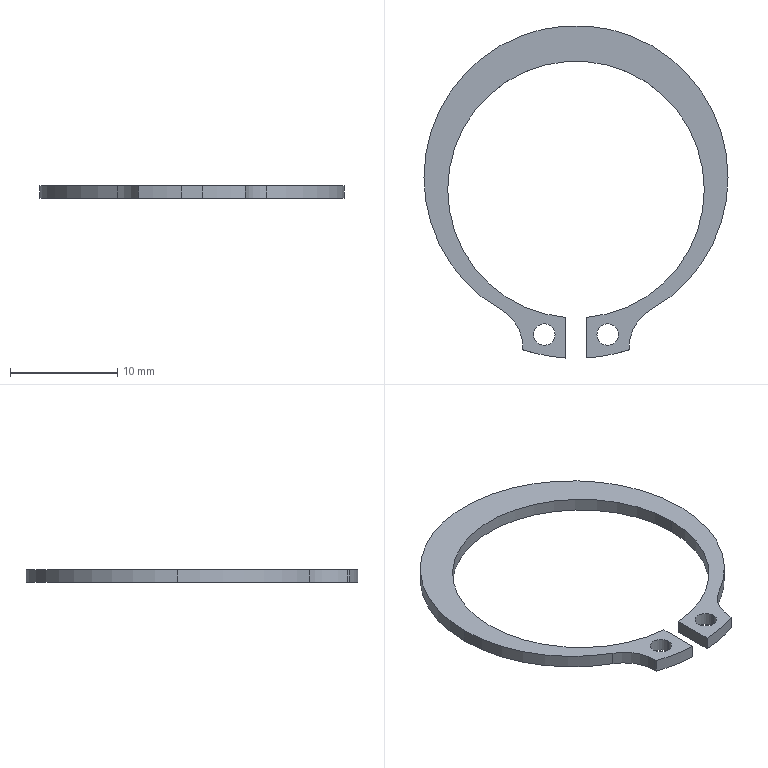Part | SolidWorks | features BaseBody 1 | 1 solid | 20 faces | box 28.327 x 30.963 x 1.2 mm | volume 236.217 mm3 | cylinder 14 | plane 6 | commonest cylinder face diameters 2 x4 23.9 x3 28.327 x3 8 x2 31.443 x2
STEP:
#1=CARTESIAN_POINT('',(4.9,-1.605,1.2));
#2=VERTEX_POINT('',#1);
#3=CARTESIAN_POINT('',(2.9,-1.605,1.2));
#4=VERTEX_POINT('',#3);
#5=CARTESIAN_POINT('',(3.9,-1.605,1.2));
#6=DIRECTION('',(0.,0.,-1.));
#7=DIRECTION('',(-1.,0.,0.));
#8=AXIS2_PLACEMENT_3D('',#5,#6,#7);
#9=CIRCLE('',#8,1.);
#10=EDGE_CURVE('',#2,#4,#9,.T.);
#11=ORIENTED_EDGE('',*,*,#10,.F.);
#12=CARTESIAN_POINT('',(4.9,-1.605,0.));
#13=VERTEX_POINT('',#12);
#14=CARTESIAN_POINT('',(4.9,-1.605,1.2));
#15=DIRECTION('',(0.,0.,-1.));
#16=VECTOR('',#15,1000.);
#17=LINE('',#14,#16);
#18=EDGE_CURVE('',#2,#13,#17,.T.);
#19=ORIENTED_EDGE('',*,*,#18,.T.);
#20=CARTESIAN_POINT('',(2.9,-1.605,0.));
#21=VERTEX_POINT('',#20);
#22=CARTESIAN_POINT('',(3.9,-1.605,0.));
#23=DIRECTION('',(0.,0.,-1.));
#24=DIRECTION('',(-1.,0.,0.));
#25=AXIS2_PLACEMENT_3D('',#22,#23,#24);
#26=CIRCLE('',#25,1.);
#27=EDGE_CURVE('',#13,#21,#26,.T.);
#28=ORIENTED_EDGE('',*,*,#27,.T.);
#29=CARTESIAN_POINT('',(2.9,-1.605,1.2));
#30=DIRECTION('',(0.,0.,-1.));
#31=VECTOR('',#30,1000.);
#32=LINE('',#29,#31);
#33=EDGE_CURVE('',#4,#21,#32,.T.);
#34=ORIENTED_EDGE('',*,*,#33,.F.);
#35=EDGE_LOOP('',(#11,#19,#28,#34));
#36=FACE_OUTER_BOUND('',#35,.T.);
#37=CARTESIAN_POINT('',(3.9,-1.605,1.2));
#38=DIRECTION('',(0.,0.,-1.));
#39=DIRECTION('',(-1.,0.,0.));
#40=AXIS2_PLACEMENT_3D('',#37,#38,#39);
#41=CYLINDRICAL_SURFACE('',#40,1.);
#42=ADVANCED_FACE('',(#36),#41,.F.);
#43=CARTESIAN_POINT('',(-1.,-1.605,0.));
#44=VERTEX_POINT('',#43);
#45=CARTESIAN_POINT('',(-3.,-1.605,0.));
#46=VERTEX_POINT('',#45);
#47=CARTESIAN_POINT('',(-2.,-1.605,0.));
#48=DIRECTION('',(0.,0.,-1.));
#49=DIRECTION('',(1.,0.,0.));
#50=AXIS2_PLACEMENT_3D('',#47,#48,#49);
#51=CIRCLE('',#50,1.);
#52=EDGE_CURVE('',#44,#46,#51,.T.);
#53=ORIENTED_EDGE('',*,*,#52,.T.);
#54=CARTESIAN_POINT('',(-3.,-1.605,1.2));
#55=VERTEX_POINT('',#54);
#56=CARTESIAN_POINT('',(-3.,-1.605,1.2));
#57=DIRECTION('',(0.,0.,1.));
#58=VECTOR('',#57,1000.);
#59=LINE('',#56,#58);
#60=EDGE_CURVE('',#46,#55,#59,.T.);
#61=ORIENTED_EDGE('',*,*,#60,.T.);
#62=CARTESIAN_POINT('',(-1.,-1.605,1.2));
#63=VERTEX_POINT('',#62);
#64=CARTESIAN_POINT('',(-2.,-1.605,1.2));
#65=DIRECTION('',(0.,0.,-1.));
#66=DIRECTION('',(1.,0.,0.));
#67=AXIS2_PLACEMENT_3D('',#64,#65,#66);
#68=CIRCLE('',#67,1.);
#69=EDGE_CURVE('',#63,#55,#68,.T.);
#70=ORIENTED_EDGE('',*,*,#69,.F.);
#71=CARTESIAN_POINT('',(-1.,-1.605,1.2));
#72=DIRECTION('',(0.,0.,1.));
#73=VECTOR('',#72,1000.);
#74=LINE('',#71,#73);
#75=EDGE_CURVE('',#44,#63,#74,.T.);
#76=ORIENTED_EDGE('',*,*,#75,.F.);
#77=EDGE_LOOP('',(#53,#61,#70,#76));
#78=FACE_OUTER_BOUND('',#77,.T.);
#79=CARTESIAN_POINT('',(-2.,-1.605,1.2));
#80=DIRECTION('',(0.,0.,1.));
#81=DIRECTION('',(1.,0.,0.));
#82=AXIS2_PLACEMENT_3D('',#79,#80,#81);
#83=CYLINDRICAL_SURFACE('',#82,1.);
#84=ADVANCED_FACE('',(#78),#83,.F.);
#85=CARTESIAN_POINT('',(15.113,13.019,0.));
#86=VERTEX_POINT('',#85);
#87=CARTESIAN_POINT('',(-13.213,13.019,0.));
#88=VERTEX_POINT('',#87);
#89=CARTESIAN_POINT('',(0.95,13.019,0.));
#90=DIRECTION('',(0.,0.,1.));
#91=DIRECTION('',(1.,0.,0.));
#92=AXIS2_PLACEMENT_3D('',#89,#90,#91);
#93=CIRCLE('',#92,14.163);
#94=EDGE_CURVE('',#86,#88,#93,.T.);
#95=ORIENTED_EDGE('',*,*,#94,.T.);
#96=CARTESIAN_POINT('',(-13.213,13.019,1.2));
#97=VERTEX_POINT('',#96);
#98=CARTESIAN_POINT('',(-13.213,13.019,0.));
#99=DIRECTION('',(0.,0.,1.));
#100=VECTOR('',#99,1000.);
#101=LINE('',#98,#100);
#102=EDGE_CURVE('',#88,#97,#101,.T.);
#103=ORIENTED_EDGE('',*,*,#102,.T.);
#104=CARTESIAN_POINT('',(15.113,13.019,1.2));
#105=VERTEX_POINT('',#104);
#106=CARTESIAN_POINT('',(0.95,13.019,1.2));
#107=DIRECTION('',(0.,0.,-1.));
#108=DIRECTION('',(1.,0.,0.));
#109=AXIS2_PLACEMENT_3D('',#106,#107,#108);
#110=CIRCLE('',#109,14.163);
#111=EDGE_CURVE('',#97,#105,#110,.T.);
#112=ORIENTED_EDGE('',*,*,#111,.T.);
#113=CARTESIAN_POINT('',(15.113,13.019,0.));
#114=DIRECTION('',(0.,0.,1.));
#115=VECTOR('',#114,1000.);
#116=LINE('',#113,#115);
#117=EDGE_CURVE('',#86,#105,#116,.T.);
#118=ORIENTED_EDGE('',*,*,#117,.F.);
#119=EDGE_LOOP('',(#95,#103,#112,#118));
#120=FACE_OUTER_BOUND('',#119,.T.);
#121=CARTESIAN_POINT('',(0.95,13.019,0.));
#122=DIRECTION('',(0.,0.,1.));
#123=DIRECTION('',(1.,0.,0.));
#124=AXIS2_PLACEMENT_3D('',#121,#122,#123);
#125=CYLINDRICAL_SURFACE('',#124,14.163);
#126=ADVANCED_FACE('',(#120),#125,.T.);
#127=CARTESIAN_POINT('',(7.929,0.6943,0.));
#128=VERTEX_POINT('',#127);
#129=CARTESIAN_POINT('',(0.95,13.019,0.));
#130=DIRECTION('',(0.,0.,1.));
#131=DIRECTION('',(1.,0.,0.));
#132=AXIS2_PLACEMENT_3D('',#129,#130,#131);
#133=CIRCLE('',#132,14.163);
#134=EDGE_CURVE('',#128,#86,#133,.T.);
#135=ORIENTED_EDGE('',*,*,#134,.T.);
#136=ORIENTED_EDGE('',*,*,#117,.T.);
#137=CARTESIAN_POINT('',(7.929,0.6943,1.2));
#138=VERTEX_POINT('',#137);
#139=CARTESIAN_POINT('',(0.95,13.019,1.2));
#140=DIRECTION('',(0.,0.,-1.));
#141=DIRECTION('',(1.,0.,0.));
#142=AXIS2_PLACEMENT_3D('',#139,#140,#141);
#143=CIRCLE('',#142,14.163);
#144=EDGE_CURVE('',#105,#138,#143,.T.);
#145=ORIENTED_EDGE('',*,*,#144,.T.);
#146=CARTESIAN_POINT('',(7.929,0.6943,0.));
#147=DIRECTION('',(0.,0.,-1.));
#148=VECTOR('',#147,1000.);
#149=LINE('',#146,#148);
#150=EDGE_CURVE('',#138,#128,#149,.T.);
#151=ORIENTED_EDGE('',*,*,#150,.T.);
#152=EDGE_LOOP('',(#135,#136,#145,#151));
#153=FACE_OUTER_BOUND('',#152,.T.);
#154=CARTESIAN_POINT('',(0.95,13.019,0.));
#155=DIRECTION('',(0.,0.,1.));
#156=DIRECTION('',(1.,0.,0.));
#157=AXIS2_PLACEMENT_3D('',#154,#155,#156);
#158=CYLINDRICAL_SURFACE('',#157,14.163);
#159=ADVANCED_FACE('',(#153),#158,.T.);
#160=CARTESIAN_POINT('',(0.,0.,0.));
#161=VERTEX_POINT('',#160);
#162=CARTESIAN_POINT('',(-11.,11.912,0.));
#163=VERTEX_POINT('',#162);
#164=CARTESIAN_POINT('',(0.95,11.912,0.));
#165=DIRECTION('',(0.,0.,-1.));
#166=DIRECTION('',(1.,0.,0.));
#167=AXIS2_PLACEMENT_3D('',#164,#165,#166);
#168=CIRCLE('',#167,11.95);
#169=EDGE_CURVE('',#161,#163,#168,.T.);
#170=ORIENTED_EDGE('',*,*,#169,.T.);
#171=CARTESIAN_POINT('',(-11.,11.912,1.2));
#172=VERTEX_POINT('',#171);
#173=CARTESIAN_POINT('',(-11.,11.912,0.));
#174=DIRECTION('',(0.,0.,1.));
#175=VECTOR('',#174,1000.);
#176=LINE('',#173,#175);
#177=EDGE_CURVE('',#163,#172,#176,.T.);
#178=ORIENTED_EDGE('',*,*,#177,.T.);
#179=CARTESIAN_POINT('',(0.,0.,1.2));
#180=VERTEX_POINT('',#179);
#181=CARTESIAN_POINT('',(0.95,11.912,1.2));
#182=DIRECTION('',(0.,0.,-1.));
#183=DIRECTION('',(1.,0.,0.));
#184=AXIS2_PLACEMENT_3D('',#181,#182,#183);
#185=CIRCLE('',#184,11.95);
#186=EDGE_CURVE('',#180,#172,#185,.T.);
#187=ORIENTED_EDGE('',*,*,#186,.F.);
#188=CARTESIAN_POINT('',(0.,0.,0.));
#189=DIRECTION('',(0.,0.,1.));
#190=VECTOR('',#189,1000.);
#191=LINE('',#188,#190);
#192=EDGE_CURVE('',#161,#180,#191,.T.);
#193=ORIENTED_EDGE('',*,*,#192,.F.);
#194=EDGE_LOOP('',(#170,#178,#187,#193));
#195=FACE_OUTER_BOUND('',#194,.T.);
#196=CARTESIAN_POINT('',(0.95,11.912,0.));
#197=DIRECTION('',(0.,0.,1.));
#198=DIRECTION('',(1.,0.,0.));
#199=AXIS2_PLACEMENT_3D('',#196,#197,#198);
#200=CYLINDRICAL_SURFACE('',#199,11.95);
#201=ADVANCED_FACE('',(#195),#200,.F.);
#202=ORIENTED_EDGE('',*,*,#177,.F.);
#203=CARTESIAN_POINT('',(12.9,11.912,0.));
#204=VERTEX_POINT('',#203);
#205=CARTESIAN_POINT('',(0.95,11.912,0.));
#206=DIRECTION('',(0.,0.,-1.));
#207=DIRECTION('',(1.,0.,0.));
#208=AXIS2_PLACEMENT_3D('',#205,#206,#207);
#209=CIRCLE('',#208,11.95);
#210=EDGE_CURVE('',#163,#204,#209,.T.);
#211=ORIENTED_EDGE('',*,*,#210,.T.);
#212=CARTESIAN_POINT('',(12.9,11.912,1.2));
#213=VERTEX_POINT('',#212);
#214=CARTESIAN_POINT('',(12.9,11.912,0.));
#215=DIRECTION('',(0.,0.,1.));
#216=VECTOR('',#215,1000.);
#217=LINE('',#214,#216);
#218=EDGE_CURVE('',#204,#213,#217,.T.);
#219=ORIENTED_EDGE('',*,*,#218,.T.);
#220=CARTESIAN_POINT('',(0.95,11.912,1.2));
#221=DIRECTION('',(0.,0.,-1.));
#222=DIRECTION('',(1.,0.,0.));
#223=AXIS2_PLACEMENT_3D('',#220,#221,#222);
#224=CIRCLE('',#223,11.95);
#225=EDGE_CURVE('',#172,#213,#224,.T.);
#226=ORIENTED_EDGE('',*,*,#225,.F.);
#227=EDGE_LOOP('',(#202,#211,#219,#226));
#228=FACE_OUTER_BOUND('',#227,.T.);
#229=CARTESIAN_POINT('',(0.95,11.912,0.));
#230=DIRECTION('',(0.,0.,1.));
#231=DIRECTION('',(1.,0.,0.));
#232=AXIS2_PLACEMENT_3D('',#229,#230,#231);
#233=CYLINDRICAL_SURFACE('',#232,11.95);
#234=ADVANCED_FACE('',(#228),#233,.F.);
#235=CARTESIAN_POINT('',(3.9,-1.605,0.));
#236=DIRECTION('',(0.,0.,-1.));
#237=DIRECTION('',(-1.,0.,0.));
#238=AXIS2_PLACEMENT_3D('',#235,#236,#237);
#239=CIRCLE('',#238,1.);
#240=EDGE_CURVE('',#21,#13,#239,.T.);
#241=ORIENTED_EDGE('',*,*,#240,.F.);
#242=ORIENTED_EDGE('',*,*,#27,.F.);
#243=EDGE_LOOP('',(#241,#242));
#244=FACE_BOUND('',#243,.T.);
#245=ORIENTED_EDGE('',*,*,#52,.F.);
#246=CARTESIAN_POINT('',(-2.,-1.605,0.));
#247=DIRECTION('',(0.,0.,-1.));
#248=DIRECTION('',(1.,0.,0.));
#249=AXIS2_PLACEMENT_3D('',#246,#247,#248);
#250=CIRCLE('',#249,1.);
#251=EDGE_CURVE('',#46,#44,#250,.T.);
#252=ORIENTED_EDGE('',*,*,#251,.F.);
#253=EDGE_LOOP('',(#245,#252));
#254=FACE_BOUND('',#253,.T.);
#255=CARTESIAN_POINT('',(-4.,-3.01,0.));
#256=VERTEX_POINT('',#255);
#257=CARTESIAN_POINT('',(0.,-3.781,0.));
#258=VERTEX_POINT('',#257);
#259=CARTESIAN_POINT('',(0.95,11.912,0.));
#260=DIRECTION('',(0.,0.,1.));
#261=DIRECTION('',(1.,0.,0.));
#262=AXIS2_PLACEMENT_3D('',#259,#260,#261);
#263=CIRCLE('',#262,15.722);
#264=EDGE_CURVE('',#256,#258,#263,.T.);
#265=ORIENTED_EDGE('',*,*,#264,.F.);
#266=CARTESIAN_POINT('',(-4.,-2.786,0.));
#267=VERTEX_POINT('',#266);
#268=CARTESIAN_POINT('',(-4.,0.,0.));
#269=DIRECTION('',(0.,-1.,0.));
#270=VECTOR('',#269,1000.);
#271=LINE('',#268,#270);
#272=EDGE_CURVE('',#267,#256,#271,.T.);
#273=ORIENTED_EDGE('',*,*,#272,.F.);
#274=CARTESIAN_POINT('',(-6.029,0.6943,0.));
#275=VERTEX_POINT('',#274);
#276=CARTESIAN_POINT('',(-8.,-2.786,0.));
#277=DIRECTION('',(0.,0.,-1.));
#278=DIRECTION('',(1.,0.,0.));
#279=AXIS2_PLACEMENT_3D('',#276,#277,#278);
#280=CIRCLE('',#279,4.);
#281=EDGE_CURVE('',#275,#267,#280,.T.);
#282=ORIENTED_EDGE('',*,*,#281,.F.);
#283=CARTESIAN_POINT('',(0.95,13.019,0.));
#284=DIRECTION('',(0.,0.,1.));
#285=DIRECTION('',(1.,0.,0.));
#286=AXIS2_PLACEMENT_3D('',#283,#284,#285);
#287=CIRCLE('',#286,14.163);
#288=EDGE_CURVE('',#88,#275,#287,.T.);
#289=ORIENTED_EDGE('',*,*,#288,.F.);
#290=ORIENTED_EDGE('',*,*,#94,.F.);
#291=ORIENTED_EDGE('',*,*,#134,.F.);
#292=CARTESIAN_POINT('',(5.9,-2.786,0.));
#293=VERTEX_POINT('',#292);
#294=CARTESIAN_POINT('',(9.9,-2.786,0.));
#295=DIRECTION('',(0.,0.,-1.));
#296=DIRECTION('',(1.,0.,0.));
#297=AXIS2_PLACEMENT_3D('',#294,#295,#296);
#298=CIRCLE('',#297,4.);
#299=EDGE_CURVE('',#293,#128,#298,.T.);
#300=ORIENTED_EDGE('',*,*,#299,.F.);
#301=CARTESIAN_POINT('',(5.9,-3.01,0.));
#302=VERTEX_POINT('',#301);
#303=CARTESIAN_POINT('',(5.9,0.,0.));
#304=DIRECTION('',(0.,1.,0.));
#305=VECTOR('',#304,1000.);
#306=LINE('',#303,#305);
#307=EDGE_CURVE('',#302,#293,#306,.T.);
#308=ORIENTED_EDGE('',*,*,#307,.F.);
#309=CARTESIAN_POINT('',(1.9,-3.781,0.));
#310=VERTEX_POINT('',#309);
#311=CARTESIAN_POINT('',(0.95,11.912,0.));
#312=DIRECTION('',(0.,0.,1.));
#313=DIRECTION('',(1.,0.,0.));
#314=AXIS2_PLACEMENT_3D('',#311,#312,#313);
#315=CIRCLE('',#314,15.722);
#316=EDGE_CURVE('',#310,#302,#315,.T.);
#317=ORIENTED_EDGE('',*,*,#316,.F.);
#318=CARTESIAN_POINT('',(1.9,0.,0.));
#319=VERTEX_POINT('',#318);
#320=CARTESIAN_POINT('',(1.9,0.,0.));
#321=DIRECTION('',(0.,-1.,0.));
#322=VECTOR('',#321,1000.);
#323=LINE('',#320,#322);
#324=EDGE_CURVE('',#319,#310,#323,.T.);
#325=ORIENTED_EDGE('',*,*,#324,.F.);
#326=CARTESIAN_POINT('',(0.95,11.912,0.));
#327=DIRECTION('',(0.,0.,-1.));
#328=DIRECTION('',(1.,0.,0.));
#329=AXIS2_PLACEMENT_3D('',#326,#327,#328);
#330=CIRCLE('',#329,11.95);
#331=EDGE_CURVE('',#204,#319,#330,.T.);
#332=ORIENTED_EDGE('',*,*,#331,.F.);
#333=ORIENTED_EDGE('',*,*,#210,.F.);
#334=ORIENTED_EDGE('',*,*,#169,.F.);
#335=CARTESIAN_POINT('',(0.,0.,0.));
#336=DIRECTION('',(0.,1.,0.));
#337=VECTOR('',#336,1000.);
#338=LINE('',#335,#337);
#339=EDGE_CURVE('',#258,#161,#338,.T.);
#340=ORIENTED_EDGE('',*,*,#339,.F.);
#341=EDGE_LOOP('',(#265,#273,#282,#289,#290,#291,#300,#308,#317,#325,#332,#333,#334,#340));
#342=FACE_OUTER_BOUND('',#341,.T.);
#343=CARTESIAN_POINT('',(0.,0.,0.));
#344=DIRECTION('',(0.,0.,1.));
#345=DIRECTION('',(1.,0.,0.));
#346=AXIS2_PLACEMENT_3D('',#343,#344,#345);
#347=PLANE('',#346);
#348=ADVANCED_FACE('',(#244,#254,#342),#347,.F.);
#349=ORIENTED_EDGE('',*,*,#18,.F.);
#350=CARTESIAN_POINT('',(3.9,-1.605,1.2));
#351=DIRECTION('',(0.,0.,-1.));
#352=DIRECTION('',(-1.,0.,0.));
#353=AXIS2_PLACEMENT_3D('',#350,#351,#352);
#354=CIRCLE('',#353,1.);
#355=EDGE_CURVE('',#4,#2,#354,.T.);
#356=ORIENTED_EDGE('',*,*,#355,.F.);
#357=ORIENTED_EDGE('',*,*,#33,.T.);
#358=ORIENTED_EDGE('',*,*,#240,.T.);
#359=EDGE_LOOP('',(#349,#356,#357,#358));
#360=FACE_OUTER_BOUND('',#359,.T.);
#361=CARTESIAN_POINT('',(3.9,-1.605,1.2));
#362=DIRECTION('',(0.,0.,-1.));
#363=DIRECTION('',(-1.,0.,0.));
#364=AXIS2_PLACEMENT_3D('',#361,#362,#363);
#365=CYLINDRICAL_SURFACE('',#364,1.);
#366=ADVANCED_FACE('',(#360),#365,.F.);
#367=ORIENTED_EDGE('',*,*,#60,.F.);
#368=ORIENTED_EDGE('',*,*,#251,.T.);
#369=ORIENTED_EDGE('',*,*,#75,.T.);
#370=CARTESIAN_POINT('',(-2.,-1.605,1.2));
#371=DIRECTION('',(0.,0.,-1.));
#372=DIRECTION('',(1.,0.,0.));
#373=AXIS2_PLACEMENT_3D('',#370,#371,#372);
#374=CIRCLE('',#373,1.);
#375=EDGE_CURVE('',#55,#63,#374,.T.);
#376=ORIENTED_EDGE('',*,*,#375,.F.);
#377=EDGE_LOOP('',(#367,#368,#369,#376));
#378=FACE_OUTER_BOUND('',#377,.T.);
#379=CARTESIAN_POINT('',(-2.,-1.605,1.2));
#380=DIRECTION('',(0.,0.,1.));
#381=DIRECTION('',(1.,0.,0.));
#382=AXIS2_PLACEMENT_3D('',#379,#380,#381);
#383=CYLINDRICAL_SURFACE('',#382,1.);
#384=ADVANCED_FACE('',(#378),#383,.F.);
#385=CARTESIAN_POINT('',(0.,-3.781,1.2));
#386=VERTEX_POINT('',#385);
#387=CARTESIAN_POINT('',(0.,-3.781,0.));
#388=DIRECTION('',(0.,0.,-1.));
#389=VECTOR('',#388,1000.);
#390=LINE('',#387,#389);
#391=EDGE_CURVE('',#386,#258,#390,.T.);
#392=ORIENTED_EDGE('',*,*,#391,.T.);
#393=ORIENTED_EDGE('',*,*,#339,.T.);
#394=ORIENTED_EDGE('',*,*,#192,.T.);
#395=CARTESIAN_POINT('',(0.,-3.781,1.2));
#396=DIRECTION('',(0.,-1.,0.));
#397=VECTOR('',#396,1000.);
#398=LINE('',#395,#397);
#399=EDGE_CURVE('',#180,#386,#398,.T.);
#400=ORIENTED_EDGE('',*,*,#399,.T.);
#401=EDGE_LOOP('',(#392,#393,#394,#400));
#402=FACE_OUTER_BOUND('',#401,.T.);
#403=CARTESIAN_POINT('',(0.,-3.781,0.));
#404=DIRECTION('',(1.,0.,0.));
#405=DIRECTION('',(0.,0.,-1.));
#406=AXIS2_PLACEMENT_3D('',#403,#404,#405);
#407=PLANE('',#406);
#408=ADVANCED_FACE('',(#402),#407,.T.);
#409=CARTESIAN_POINT('',(-4.,-3.01,1.2));
#410=VERTEX_POINT('',#409);
#411=CARTESIAN_POINT('',(-4.,-3.01,0.));
#412=DIRECTION('',(0.,0.,-1.));
#413=VECTOR('',#412,1000.);
#414=LINE('',#411,#413);
#415=EDGE_CURVE('',#410,#256,#414,.T.);
#416=ORIENTED_EDGE('',*,*,#415,.T.);
#417=ORIENTED_EDGE('',*,*,#264,.T.);
#418=ORIENTED_EDGE('',*,*,#391,.F.);
#419=CARTESIAN_POINT('',(0.95,11.912,1.2));
#420=DIRECTION('',(0.,0.,-1.));
#421=DIRECTION('',(1.,0.,0.));
#422=AXIS2_PLACEMENT_3D('',#419,#420,#421);
#423=CIRCLE('',#422,15.722);
#424=EDGE_CURVE('',#386,#410,#423,.T.);
#425=ORIENTED_EDGE('',*,*,#424,.T.);
#426=EDGE_LOOP('',(#416,#417,#418,#425));
#427=FACE_OUTER_BOUND('',#426,.T.);
#428=CARTESIAN_POINT('',(0.95,11.912,0.));
#429=DIRECTION('',(0.,0.,1.));
#430=DIRECTION('',(1.,0.,0.));
#431=AXIS2_PLACEMENT_3D('',#428,#429,#430);
#432=CYLINDRICAL_SURFACE('',#431,15.722);
#433=ADVANCED_FACE('',(#427),#432,.T.);
#434=CARTESIAN_POINT('',(-4.,-2.786,1.2));
#435=VERTEX_POINT('',#434);
#436=CARTESIAN_POINT('',(-4.,-2.786,0.));
#437=DIRECTION('',(0.,0.,-1.));
#438=VECTOR('',#437,1000.);
#439=LINE('',#436,#438);
#440=EDGE_CURVE('',#435,#267,#439,.T.);
#441=ORIENTED_EDGE('',*,*,#440,.T.);
#442=ORIENTED_EDGE('',*,*,#272,.T.);
#443=ORIENTED_EDGE('',*,*,#415,.F.);
#444=CARTESIAN_POINT('',(-4.,-2.786,1.2));
#445=DIRECTION('',(0.,1.,0.));
#446=VECTOR('',#445,1000.);
#447=LINE('',#444,#446);
#448=EDGE_CURVE('',#410,#435,#447,.T.);
#449=ORIENTED_EDGE('',*,*,#448,.T.);
#450=EDGE_LOOP('',(#441,#442,#443,#449));
#451=FACE_OUTER_BOUND('',#450,.T.);
#452=CARTESIAN_POINT('',(-4.,-2.786,0.));
#453=DIRECTION('',(-1.,0.,0.));
#454=DIRECTION('',(0.,0.,1.));
#455=AXIS2_PLACEMENT_3D('',#452,#453,#454);
#456=PLANE('',#455);
#457=ADVANCED_FACE('',(#451),#456,.T.);
#458=CARTESIAN_POINT('',(-6.029,0.6943,1.2));
#459=VERTEX_POINT('',#458);
#460=CARTESIAN_POINT('',(-8.,-2.786,1.2));
#461=DIRECTION('',(0.,0.,-1.));
#462=DIRECTION('',(1.,0.,0.));
#463=AXIS2_PLACEMENT_3D('',#460,#461,#462);
#464=CIRCLE('',#463,4.);
#465=EDGE_CURVE('',#459,#435,#464,.T.);
#466=ORIENTED_EDGE('',*,*,#465,.F.);
#467=CARTESIAN_POINT('',(-6.029,0.6943,0.));
#468=DIRECTION('',(0.,0.,1.));
#469=VECTOR('',#468,1000.);
#470=LINE('',#467,#469);
#471=EDGE_CURVE('',#275,#459,#470,.T.);
#472=ORIENTED_EDGE('',*,*,#471,.F.);
#473=ORIENTED_EDGE('',*,*,#281,.T.);
#474=ORIENTED_EDGE('',*,*,#440,.F.);
#475=EDGE_LOOP('',(#466,#472,#473,#474));
#476=FACE_OUTER_BOUND('',#475,.T.);
#477=CARTESIAN_POINT('',(-8.,-2.786,0.));
#478=DIRECTION('',(0.,0.,1.));
#479=DIRECTION('',(1.,0.,0.));
#480=AXIS2_PLACEMENT_3D('',#477,#478,#479);
#481=CYLINDRICAL_SURFACE('',#480,4.);
#482=ADVANCED_FACE('',(#476),#481,.F.);
#483=ORIENTED_EDGE('',*,*,#102,.F.);
#484=ORIENTED_EDGE('',*,*,#288,.T.);
#485=ORIENTED_EDGE('',*,*,#471,.T.);
#486=CARTESIAN_POINT('',(0.95,13.019,1.2));
#487=DIRECTION('',(0.,0.,-1.));
#488=DIRECTION('',(1.,0.,0.));
#489=AXIS2_PLACEMENT_3D('',#486,#487,#488);
#490=CIRCLE('',#489,14.163);
#491=EDGE_CURVE('',#459,#97,#490,.T.);
#492=ORIENTED_EDGE('',*,*,#491,.T.);
#493=EDGE_LOOP('',(#483,#484,#485,#492));
#494=FACE_OUTER_BOUND('',#493,.T.);
#495=CARTESIAN_POINT('',(0.95,13.019,0.));
#496=DIRECTION('',(0.,0.,1.));
#497=DIRECTION('',(1.,0.,0.));
#498=AXIS2_PLACEMENT_3D('',#495,#496,#497);
#499=CYLINDRICAL_SURFACE('',#498,14.163);
#500=ADVANCED_FACE('',(#494),#499,.T.);
#501=CARTESIAN_POINT('',(5.9,-2.786,1.2));
#502=VERTEX_POINT('',#501);
#503=CARTESIAN_POINT('',(9.9,-2.786,1.2));
#504=DIRECTION('',(0.,0.,-1.));
#505=DIRECTION('',(1.,0.,0.));
#506=AXIS2_PLACEMENT_3D('',#503,#504,#505);
#507=CIRCLE('',#506,4.);
#508=EDGE_CURVE('',#502,#138,#507,.T.);
#509=ORIENTED_EDGE('',*,*,#508,.F.);
#510=CARTESIAN_POINT('',(5.9,-2.786,0.));
#511=DIRECTION('',(0.,0.,1.));
#512=VECTOR('',#511,1000.);
#513=LINE('',#510,#512);
#514=EDGE_CURVE('',#293,#502,#513,.T.);
#515=ORIENTED_EDGE('',*,*,#514,.F.);
#516=ORIENTED_EDGE('',*,*,#299,.T.);
#517=ORIENTED_EDGE('',*,*,#150,.F.);
#518=EDGE_LOOP('',(#509,#515,#516,#517));
#519=FACE_OUTER_BOUND('',#518,.T.);
#520=CARTESIAN_POINT('',(9.9,-2.786,0.));
#521=DIRECTION('',(0.,0.,1.));
#522=DIRECTION('',(1.,0.,0.));
#523=AXIS2_PLACEMENT_3D('',#520,#521,#522);
#524=CYLINDRICAL_SURFACE('',#523,4.);
#525=ADVANCED_FACE('',(#519),#524,.F.);
#526=CARTESIAN_POINT('',(5.9,-3.01,1.2));
#527=VERTEX_POINT('',#526);
#528=CARTESIAN_POINT('',(5.9,-3.01,0.));
#529=DIRECTION('',(0.,0.,-1.));
#530=VECTOR('',#529,1000.);
#531=LINE('',#528,#530);
#532=EDGE_CURVE('',#527,#302,#531,.T.);
#533=ORIENTED_EDGE('',*,*,#532,.T.);
#534=ORIENTED_EDGE('',*,*,#307,.T.);
#535=ORIENTED_EDGE('',*,*,#514,.T.);
#536=CARTESIAN_POINT('',(5.9,-3.01,1.2));
#537=DIRECTION('',(0.,-1.,0.));
#538=VECTOR('',#537,1000.);
#539=LINE('',#536,#538);
#540=EDGE_CURVE('',#502,#527,#539,.T.);
#541=ORIENTED_EDGE('',*,*,#540,.T.);
#542=EDGE_LOOP('',(#533,#534,#535,#541));
#543=FACE_OUTER_BOUND('',#542,.T.);
#544=CARTESIAN_POINT('',(5.9,-3.01,0.));
#545=DIRECTION('',(1.,0.,0.));
#546=DIRECTION('',(0.,0.,-1.));
#547=AXIS2_PLACEMENT_3D('',#544,#545,#546);
#548=PLANE('',#547);
#549=ADVANCED_FACE('',(#543),#548,.T.);
#550=CARTESIAN_POINT('',(1.9,-3.781,1.2));
#551=VERTEX_POINT('',#550);
#552=CARTESIAN_POINT('',(1.9,-3.781,0.));
#553=DIRECTION('',(0.,0.,-1.));
#554=VECTOR('',#553,1000.);
#555=LINE('',#552,#554);
#556=EDGE_CURVE('',#551,#310,#555,.T.);
#557=ORIENTED_EDGE('',*,*,#556,.T.);
#558=ORIENTED_EDGE('',*,*,#316,.T.);
#559=ORIENTED_EDGE('',*,*,#532,.F.);
#560=CARTESIAN_POINT('',(0.95,11.912,1.2));
#561=DIRECTION('',(0.,0.,-1.));
#562=DIRECTION('',(1.,0.,0.));
#563=AXIS2_PLACEMENT_3D('',#560,#561,#562);
#564=CIRCLE('',#563,15.722);
#565=EDGE_CURVE('',#527,#551,#564,.T.);
#566=ORIENTED_EDGE('',*,*,#565,.T.);
#567=EDGE_LOOP('',(#557,#558,#559,#566));
#568=FACE_OUTER_BOUND('',#567,.T.);
#569=CARTESIAN_POINT('',(0.95,11.912,0.));
#570=DIRECTION('',(0.,0.,1.));
#571=DIRECTION('',(1.,0.,0.));
#572=AXIS2_PLACEMENT_3D('',#569,#570,#571);
#573=CYLINDRICAL_SURFACE('',#572,15.722);
#574=ADVANCED_FACE('',(#568),#573,.T.);
#575=CARTESIAN_POINT('',(1.9,0.,1.2));
#576=VERTEX_POINT('',#575);
#577=CARTESIAN_POINT('',(1.9,0.,0.));
#578=DIRECTION('',(0.,0.,-1.));
#579=VECTOR('',#578,1000.);
#580=LINE('',#577,#579);
#581=EDGE_CURVE('',#576,#319,#580,.T.);
#582=ORIENTED_EDGE('',*,*,#581,.T.);
#583=ORIENTED_EDGE('',*,*,#324,.T.);
#584=ORIENTED_EDGE('',*,*,#556,.F.);
#585=CARTESIAN_POINT('',(1.9,0.,1.2));
#586=DIRECTION('',(0.,1.,0.));
#587=VECTOR('',#586,1000.);
#588=LINE('',#585,#587);
#589=EDGE_CURVE('',#551,#576,#588,.T.);
#590=ORIENTED_EDGE('',*,*,#589,.T.);
#591=EDGE_LOOP('',(#582,#583,#584,#590));
#592=FACE_OUTER_BOUND('',#591,.T.);
#593=CARTESIAN_POINT('',(1.9,0.,0.));
#594=DIRECTION('',(-1.,0.,0.));
#595=DIRECTION('',(0.,0.,1.));
#596=AXIS2_PLACEMENT_3D('',#593,#594,#595);
#597=PLANE('',#596);
#598=ADVANCED_FACE('',(#592),#597,.T.);
#599=ORIENTED_EDGE('',*,*,#218,.F.);
#600=ORIENTED_EDGE('',*,*,#331,.T.);
#601=ORIENTED_EDGE('',*,*,#581,.F.);
#602=CARTESIAN_POINT('',(0.95,11.912,1.2));
#603=DIRECTION('',(0.,0.,-1.));
#604=DIRECTION('',(1.,0.,0.));
#605=AXIS2_PLACEMENT_3D('',#602,#603,#604);
#606=CIRCLE('',#605,11.95);
#607=EDGE_CURVE('',#213,#576,#606,.T.);
#608=ORIENTED_EDGE('',*,*,#607,.F.);
#609=EDGE_LOOP('',(#599,#600,#601,#608));
#610=FACE_OUTER_BOUND('',#609,.T.);
#611=CARTESIAN_POINT('',(0.95,11.912,0.));
#612=DIRECTION('',(0.,0.,1.));
#613=DIRECTION('',(1.,0.,0.));
#614=AXIS2_PLACEMENT_3D('',#611,#612,#613);
#615=CYLINDRICAL_SURFACE('',#614,11.95);
#616=ADVANCED_FACE('',(#610),#615,.F.);
#617=ORIENTED_EDGE('',*,*,#355,.T.);
#618=ORIENTED_EDGE('',*,*,#10,.T.);
#619=EDGE_LOOP('',(#617,#618));
#620=FACE_BOUND('',#619,.T.);
#621=ORIENTED_EDGE('',*,*,#69,.T.);
#622=ORIENTED_EDGE('',*,*,#375,.T.);
#623=EDGE_LOOP('',(#621,#622));
#624=FACE_BOUND('',#623,.T.);
#625=ORIENTED_EDGE('',*,*,#399,.F.);
#626=ORIENTED_EDGE('',*,*,#186,.T.);
#627=ORIENTED_EDGE('',*,*,#225,.T.);
#628=ORIENTED_EDGE('',*,*,#607,.T.);
#629=ORIENTED_EDGE('',*,*,#589,.F.);
#630=ORIENTED_EDGE('',*,*,#565,.F.);
#631=ORIENTED_EDGE('',*,*,#540,.F.);
#632=ORIENTED_EDGE('',*,*,#508,.T.);
#633=ORIENTED_EDGE('',*,*,#144,.F.);
#634=ORIENTED_EDGE('',*,*,#111,.F.);
#635=ORIENTED_EDGE('',*,*,#491,.F.);
#636=ORIENTED_EDGE('',*,*,#465,.T.);
#637=ORIENTED_EDGE('',*,*,#448,.F.);
#638=ORIENTED_EDGE('',*,*,#424,.F.);
#639=EDGE_LOOP('',(#625,#626,#627,#628,#629,#630,#631,#632,#633,#634,#635,#636,#637,#638));
#640=FACE_OUTER_BOUND('',#639,.T.);
#641=CARTESIAN_POINT('',(0.,0.,1.2));
#642=DIRECTION('',(0.,0.,1.));
#643=DIRECTION('',(1.,0.,0.));
#644=AXIS2_PLACEMENT_3D('',#641,#642,#643);
#645=PLANE('',#644);
#646=ADVANCED_FACE('',(#620,#624,#640),#645,.T.);
#647=CLOSED_SHELL('',(#42,#84,#126,#159,#201,#234,#348,#366,#384,#408,#433,#457,#482,#500,#525,#549,#574,#598,#616,#646));
#648=MANIFOLD_SOLID_BREP('',#647);
#649=CARTESIAN_POINT('',(0.,0.,0.));
#650=DIRECTION('',(0.,0.,1.));
#651=DIRECTION('',(1.,0.,0.));
#652=AXIS2_PLACEMENT_3D('',#649,#650,#651);
#653=(LENGTH_UNIT()NAMED_UNIT(*)SI_UNIT(.MILLI.,.METRE.));
#654=UNCERTAINTY_MEASURE_WITH_UNIT(LENGTH_MEASURE(0.00001),#653,'','');
#655=(NAMED_UNIT(*)PLANE_ANGLE_UNIT()SI_UNIT($,.RADIAN.));
#656=(NAMED_UNIT(*)SI_UNIT($,.STERADIAN.)SOLID_ANGLE_UNIT());
#657=(GEOMETRIC_REPRESENTATION_CONTEXT(3)GLOBAL_UNCERTAINTY_ASSIGNED_CONTEXT((#654))GLOBAL_UNIT_ASSIGNED_CONTEXT((#653,#655,#656))REPRESENTATION_CONTEXT('',''));
#658=ADVANCED_BREP_SHAPE_REPRESENTATION('',(#648,#652),#657);